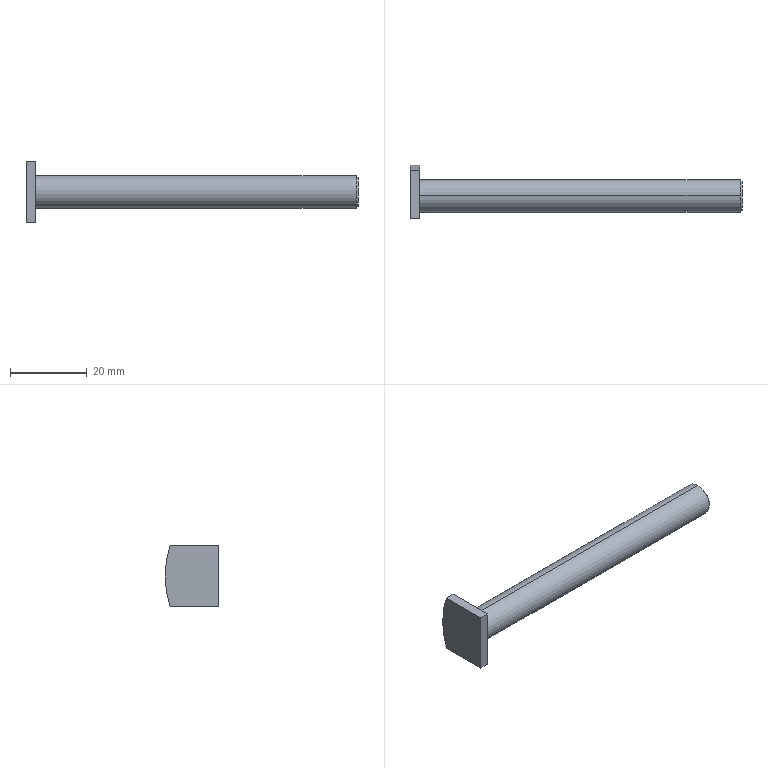Part | SolidWorks | features Chamfer 1, ICE 1, Revolution 1 | 1 solid | 11 faces | box 86.5 x 14 x 16 mm | volume 5306 mm3 | plane 6 | cylinder 3 | cone 2 | commonest cylinder face diameters 8.5 x2 50 x1
STEP:
#1=CARTESIAN_POINT('',(84.,0.,-3.75));
#2=VERTEX_POINT('',#1);
#3=CARTESIAN_POINT('',(84.,0.,3.75));
#4=VERTEX_POINT('',#3);
#5=CARTESIAN_POINT('',(84.,0.,0.));
#6=DIRECTION('',(1.,0.,0.));
#7=DIRECTION('',(0.,0.,-1.));
#8=AXIS2_PLACEMENT_3D('',#5,#6,#7);
#9=CIRCLE('',#8,3.75);
#10=EDGE_CURVE('',#2,#4,#9,.T.);
#11=ORIENTED_EDGE('',*,*,#10,.F.);
#12=CARTESIAN_POINT('',(83.5,0.,-4.25));
#13=VERTEX_POINT('',#12);
#14=CARTESIAN_POINT('',(83.5,0.,-4.25));
#15=DIRECTION('',(-0.7071,0.,-0.7071));
#16=VECTOR('',#15,1000.);
#17=LINE('',#14,#16);
#18=EDGE_CURVE('',#2,#13,#17,.T.);
#19=ORIENTED_EDGE('',*,*,#18,.T.);
#20=CARTESIAN_POINT('',(83.5,0.,4.25));
#21=VERTEX_POINT('',#20);
#22=CARTESIAN_POINT('',(83.5,0.,0.));
#23=DIRECTION('',(-1.,0.,0.));
#24=DIRECTION('',(0.,0.,-1.));
#25=AXIS2_PLACEMENT_3D('',#22,#23,#24);
#26=CIRCLE('',#25,4.25);
#27=EDGE_CURVE('',#21,#13,#26,.T.);
#28=ORIENTED_EDGE('',*,*,#27,.F.);
#29=CARTESIAN_POINT('',(83.5,0.,4.25));
#30=DIRECTION('',(-0.7071,0.,0.7071));
#31=VECTOR('',#30,1000.);
#32=LINE('',#29,#31);
#33=EDGE_CURVE('',#4,#21,#32,.T.);
#34=ORIENTED_EDGE('',*,*,#33,.F.);
#35=EDGE_LOOP('',(#11,#19,#28,#34));
#36=FACE_OUTER_BOUND('',#35,.T.);
#37=CARTESIAN_POINT('',(83.5,0.,0.));
#38=DIRECTION('',(-1.,0.,0.));
#39=DIRECTION('',(0.,0.,1.));
#40=AXIS2_PLACEMENT_3D('',#37,#38,#39);
#41=CONICAL_SURFACE('',#40,4.25,0.7854);
#42=ADVANCED_FACE('',(#36),#41,.T.);
#43=ORIENTED_EDGE('',*,*,#27,.T.);
#44=CARTESIAN_POINT('',(0.,0.,-4.25));
#45=VERTEX_POINT('',#44);
#46=CARTESIAN_POINT('',(-1.134,0.,-4.25));
#47=DIRECTION('',(-1.,0.,0.));
#48=VECTOR('',#47,1000.);
#49=LINE('',#46,#48);
#50=EDGE_CURVE('',#13,#45,#49,.T.);
#51=ORIENTED_EDGE('',*,*,#50,.T.);
#52=CARTESIAN_POINT('',(0.,0.,4.25));
#53=VERTEX_POINT('',#52);
#54=CARTESIAN_POINT('',(0.,0.,0.));
#55=DIRECTION('',(-1.,0.,0.));
#56=DIRECTION('',(0.,0.,1.));
#57=AXIS2_PLACEMENT_3D('',#54,#55,#56);
#58=CIRCLE('',#57,4.25);
#59=EDGE_CURVE('',#53,#45,#58,.T.);
#60=ORIENTED_EDGE('',*,*,#59,.F.);
#61=CARTESIAN_POINT('',(-1.134,0.,4.25));
#62=DIRECTION('',(-1.,0.,0.));
#63=VECTOR('',#62,1000.);
#64=LINE('',#61,#63);
#65=EDGE_CURVE('',#21,#53,#64,.T.);
#66=ORIENTED_EDGE('',*,*,#65,.F.);
#67=EDGE_LOOP('',(#43,#51,#60,#66));
#68=FACE_OUTER_BOUND('',#67,.T.);
#69=CARTESIAN_POINT('',(-1.134,0.,0.));
#70=DIRECTION('',(-1.,0.,0.));
#71=DIRECTION('',(0.,0.,1.));
#72=AXIS2_PLACEMENT_3D('',#69,#70,#71);
#73=CYLINDRICAL_SURFACE('',#72,4.25);
#74=ADVANCED_FACE('',(#68),#73,.T.);
#75=ORIENTED_EDGE('',*,*,#50,.F.);
#76=CARTESIAN_POINT('',(83.5,0.,0.));
#77=DIRECTION('',(-1.,0.,0.));
#78=DIRECTION('',(0.,0.,-1.));
#79=AXIS2_PLACEMENT_3D('',#76,#77,#78);
#80=CIRCLE('',#79,4.25);
#81=EDGE_CURVE('',#13,#21,#80,.T.);
#82=ORIENTED_EDGE('',*,*,#81,.T.);
#83=ORIENTED_EDGE('',*,*,#65,.T.);
#84=CARTESIAN_POINT('',(0.,0.,0.));
#85=DIRECTION('',(-1.,0.,0.));
#86=DIRECTION('',(0.,0.,1.));
#87=AXIS2_PLACEMENT_3D('',#84,#85,#86);
#88=CIRCLE('',#87,4.25);
#89=EDGE_CURVE('',#45,#53,#88,.T.);
#90=ORIENTED_EDGE('',*,*,#89,.F.);
#91=EDGE_LOOP('',(#75,#82,#83,#90));
#92=FACE_OUTER_BOUND('',#91,.T.);
#93=CARTESIAN_POINT('',(-1.134,0.,0.));
#94=DIRECTION('',(-1.,0.,0.));
#95=DIRECTION('',(0.,0.,1.));
#96=AXIS2_PLACEMENT_3D('',#93,#94,#95);
#97=CYLINDRICAL_SURFACE('',#96,4.25);
#98=ADVANCED_FACE('',(#92),#97,.T.);
#99=CARTESIAN_POINT('',(84.,0.,0.));
#100=DIRECTION('',(1.,0.,0.));
#101=DIRECTION('',(0.,0.,-1.));
#102=AXIS2_PLACEMENT_3D('',#99,#100,#101);
#103=CIRCLE('',#102,3.75);
#104=EDGE_CURVE('',#4,#2,#103,.T.);
#105=ORIENTED_EDGE('',*,*,#104,.T.);
#106=ORIENTED_EDGE('',*,*,#10,.T.);
#107=EDGE_LOOP('',(#105,#106));
#108=FACE_OUTER_BOUND('',#107,.T.);
#109=CARTESIAN_POINT('',(84.,0.,0.));
#110=DIRECTION('',(1.,0.,0.));
#111=DIRECTION('',(0.,0.,-1.));
#112=AXIS2_PLACEMENT_3D('',#109,#110,#111);
#113=PLANE('',#112);
#114=ADVANCED_FACE('',(#108),#113,.T.);
#115=ORIENTED_EDGE('',*,*,#18,.F.);
#116=ORIENTED_EDGE('',*,*,#104,.F.);
#117=ORIENTED_EDGE('',*,*,#33,.T.);
#118=ORIENTED_EDGE('',*,*,#81,.F.);
#119=EDGE_LOOP('',(#115,#116,#117,#118));
#120=FACE_OUTER_BOUND('',#119,.T.);
#121=CARTESIAN_POINT('',(83.5,0.,0.));
#122=DIRECTION('',(-1.,0.,0.));
#123=DIRECTION('',(0.,0.,1.));
#124=AXIS2_PLACEMENT_3D('',#121,#122,#123);
#125=CONICAL_SURFACE('',#124,4.25,0.7854);
#126=ADVANCED_FACE('',(#120),#125,.T.);
#127=CARTESIAN_POINT('',(0.,-6.,8.));
#128=VERTEX_POINT('',#127);
#129=CARTESIAN_POINT('',(0.,6.685,8.));
#130=VERTEX_POINT('',#129);
#131=CARTESIAN_POINT('',(0.,6.685,8.));
#132=DIRECTION('',(0.,1.,0.));
#133=VECTOR('',#132,1000.);
#134=LINE('',#131,#133);
#135=EDGE_CURVE('',#128,#130,#134,.T.);
#136=ORIENTED_EDGE('',*,*,#135,.T.);
#137=CARTESIAN_POINT('',(-2.5,6.685,8.));
#138=VERTEX_POINT('',#137);
#139=CARTESIAN_POINT('',(-2.5,6.685,8.));
#140=DIRECTION('',(1.,0.,0.));
#141=VECTOR('',#140,1000.);
#142=LINE('',#139,#141);
#143=EDGE_CURVE('',#138,#130,#142,.T.);
#144=ORIENTED_EDGE('',*,*,#143,.F.);
#145=CARTESIAN_POINT('',(-2.5,-6.,8.));
#146=VERTEX_POINT('',#145);
#147=CARTESIAN_POINT('',(-2.5,6.685,8.));
#148=DIRECTION('',(0.,1.,0.));
#149=VECTOR('',#148,1000.);
#150=LINE('',#147,#149);
#151=EDGE_CURVE('',#146,#138,#150,.T.);
#152=ORIENTED_EDGE('',*,*,#151,.F.);
#153=CARTESIAN_POINT('',(-2.5,-6.,8.));
#154=DIRECTION('',(1.,0.,0.));
#155=VECTOR('',#154,1000.);
#156=LINE('',#153,#155);
#157=EDGE_CURVE('',#146,#128,#156,.T.);
#158=ORIENTED_EDGE('',*,*,#157,.T.);
#159=EDGE_LOOP('',(#136,#144,#152,#158));
#160=FACE_OUTER_BOUND('',#159,.T.);
#161=CARTESIAN_POINT('',(-2.5,6.685,8.));
#162=DIRECTION('',(0.,0.,-1.));
#163=DIRECTION('',(0.,1.,0.));
#164=AXIS2_PLACEMENT_3D('',#161,#162,#163);
#165=PLANE('',#164);
#166=ADVANCED_FACE('',(#160),#165,.F.);
#167=CARTESIAN_POINT('',(0.,6.685,-8.));
#168=VERTEX_POINT('',#167);
#169=CARTESIAN_POINT('',(0.,-17.,0.));
#170=DIRECTION('',(-1.,0.,0.));
#171=DIRECTION('',(0.,0.,-1.));
#172=AXIS2_PLACEMENT_3D('',#169,#170,#171);
#173=CIRCLE('',#172,25.);
#174=EDGE_CURVE('',#130,#168,#173,.T.);
#175=ORIENTED_EDGE('',*,*,#174,.T.);
#176=CARTESIAN_POINT('',(-2.5,6.685,-8.));
#177=VERTEX_POINT('',#176);
#178=CARTESIAN_POINT('',(-2.5,6.685,-8.));
#179=DIRECTION('',(1.,0.,0.));
#180=VECTOR('',#179,1000.);
#181=LINE('',#178,#180);
#182=EDGE_CURVE('',#177,#168,#181,.T.);
#183=ORIENTED_EDGE('',*,*,#182,.F.);
#184=CARTESIAN_POINT('',(-2.5,-17.,0.));
#185=DIRECTION('',(-1.,0.,0.));
#186=DIRECTION('',(0.,0.,-1.));
#187=AXIS2_PLACEMENT_3D('',#184,#185,#186);
#188=CIRCLE('',#187,25.);
#189=EDGE_CURVE('',#138,#177,#188,.T.);
#190=ORIENTED_EDGE('',*,*,#189,.F.);
#191=ORIENTED_EDGE('',*,*,#143,.T.);
#192=EDGE_LOOP('',(#175,#183,#190,#191));
#193=FACE_OUTER_BOUND('',#192,.T.);
#194=CARTESIAN_POINT('',(-2.5,-17.,0.));
#195=DIRECTION('',(1.,0.,0.));
#196=DIRECTION('',(0.,0.,-1.));
#197=AXIS2_PLACEMENT_3D('',#194,#195,#196);
#198=CYLINDRICAL_SURFACE('',#197,25.);
#199=ADVANCED_FACE('',(#193),#198,.T.);
#200=CARTESIAN_POINT('',(0.,-6.,-8.));
#201=VERTEX_POINT('',#200);
#202=CARTESIAN_POINT('',(0.,6.685,-8.));
#203=DIRECTION('',(0.,-1.,0.));
#204=VECTOR('',#203,1000.);
#205=LINE('',#202,#204);
#206=EDGE_CURVE('',#168,#201,#205,.T.);
#207=ORIENTED_EDGE('',*,*,#206,.T.);
#208=CARTESIAN_POINT('',(-2.5,-6.,-8.));
#209=VERTEX_POINT('',#208);
#210=CARTESIAN_POINT('',(-2.5,-6.,-8.));
#211=DIRECTION('',(1.,0.,0.));
#212=VECTOR('',#211,1000.);
#213=LINE('',#210,#212);
#214=EDGE_CURVE('',#209,#201,#213,.T.);
#215=ORIENTED_EDGE('',*,*,#214,.F.);
#216=CARTESIAN_POINT('',(-2.5,6.685,-8.));
#217=DIRECTION('',(0.,-1.,0.));
#218=VECTOR('',#217,1000.);
#219=LINE('',#216,#218);
#220=EDGE_CURVE('',#177,#209,#219,.T.);
#221=ORIENTED_EDGE('',*,*,#220,.F.);
#222=ORIENTED_EDGE('',*,*,#182,.T.);
#223=EDGE_LOOP('',(#207,#215,#221,#222));
#224=FACE_OUTER_BOUND('',#223,.T.);
#225=CARTESIAN_POINT('',(-2.5,6.685,-8.));
#226=DIRECTION('',(0.,0.,1.));
#227=DIRECTION('',(1.,0.,0.));
#228=AXIS2_PLACEMENT_3D('',#225,#226,#227);
#229=PLANE('',#228);
#230=ADVANCED_FACE('',(#224),#229,.F.);
#231=CARTESIAN_POINT('',(0.,-6.,-8.));
#232=DIRECTION('',(0.,0.,1.));
#233=VECTOR('',#232,1000.);
#234=LINE('',#231,#233);
#235=EDGE_CURVE('',#201,#128,#234,.T.);
#236=ORIENTED_EDGE('',*,*,#235,.T.);
#237=ORIENTED_EDGE('',*,*,#157,.F.);
#238=CARTESIAN_POINT('',(-2.5,-6.,-8.));
#239=DIRECTION('',(0.,0.,1.));
#240=VECTOR('',#239,1000.);
#241=LINE('',#238,#240);
#242=EDGE_CURVE('',#209,#146,#241,.T.);
#243=ORIENTED_EDGE('',*,*,#242,.F.);
#244=ORIENTED_EDGE('',*,*,#214,.T.);
#245=EDGE_LOOP('',(#236,#237,#243,#244));
#246=FACE_OUTER_BOUND('',#245,.T.);
#247=CARTESIAN_POINT('',(-2.5,-6.,-8.));
#248=DIRECTION('',(0.,1.,0.));
#249=DIRECTION('',(0.,0.,1.));
#250=AXIS2_PLACEMENT_3D('',#247,#248,#249);
#251=PLANE('',#250);
#252=ADVANCED_FACE('',(#246),#251,.F.);
#253=ORIENTED_EDGE('',*,*,#151,.T.);
#254=ORIENTED_EDGE('',*,*,#189,.T.);
#255=ORIENTED_EDGE('',*,*,#220,.T.);
#256=ORIENTED_EDGE('',*,*,#242,.T.);
#257=EDGE_LOOP('',(#253,#254,#255,#256));
#258=FACE_OUTER_BOUND('',#257,.T.);
#259=CARTESIAN_POINT('',(-2.5,-17.,0.));
#260=DIRECTION('',(1.,0.,0.));
#261=DIRECTION('',(0.,0.,-1.));
#262=AXIS2_PLACEMENT_3D('',#259,#260,#261);
#263=PLANE('',#262);
#264=ADVANCED_FACE('',(#258),#263,.F.);
#265=ORIENTED_EDGE('',*,*,#59,.T.);
#266=ORIENTED_EDGE('',*,*,#89,.T.);
#267=EDGE_LOOP('',(#265,#266));
#268=FACE_BOUND('',#267,.T.);
#269=ORIENTED_EDGE('',*,*,#135,.F.);
#270=ORIENTED_EDGE('',*,*,#235,.F.);
#271=ORIENTED_EDGE('',*,*,#206,.F.);
#272=ORIENTED_EDGE('',*,*,#174,.F.);
#273=EDGE_LOOP('',(#269,#270,#271,#272));
#274=FACE_OUTER_BOUND('',#273,.T.);
#275=CARTESIAN_POINT('',(0.,-17.,0.));
#276=DIRECTION('',(1.,0.,0.));
#277=DIRECTION('',(0.,0.,-1.));
#278=AXIS2_PLACEMENT_3D('',#275,#276,#277);
#279=PLANE('',#278);
#280=ADVANCED_FACE('',(#268,#274),#279,.T.);
#281=CLOSED_SHELL('',(#42,#74,#98,#114,#126,#166,#199,#230,#252,#264,#280));
#282=MANIFOLD_SOLID_BREP('',#281);
#283=CARTESIAN_POINT('',(0.,0.,0.));
#284=DIRECTION('',(0.,0.,1.));
#285=DIRECTION('',(1.,0.,0.));
#286=AXIS2_PLACEMENT_3D('',#283,#284,#285);
#287=(LENGTH_UNIT()NAMED_UNIT(*)SI_UNIT(.MILLI.,.METRE.));
#288=UNCERTAINTY_MEASURE_WITH_UNIT(LENGTH_MEASURE(0.00001),#287,'','');
#289=(NAMED_UNIT(*)PLANE_ANGLE_UNIT()SI_UNIT($,.RADIAN.));
#290=(NAMED_UNIT(*)SI_UNIT($,.STERADIAN.)SOLID_ANGLE_UNIT());
#291=(GEOMETRIC_REPRESENTATION_CONTEXT(3)GLOBAL_UNCERTAINTY_ASSIGNED_CONTEXT((#288))GLOBAL_UNIT_ASSIGNED_CONTEXT((#287,#289,#290))REPRESENTATION_CONTEXT('',''));
#292=ADVANCED_BREP_SHAPE_REPRESENTATION('',(#282,#286),#291);